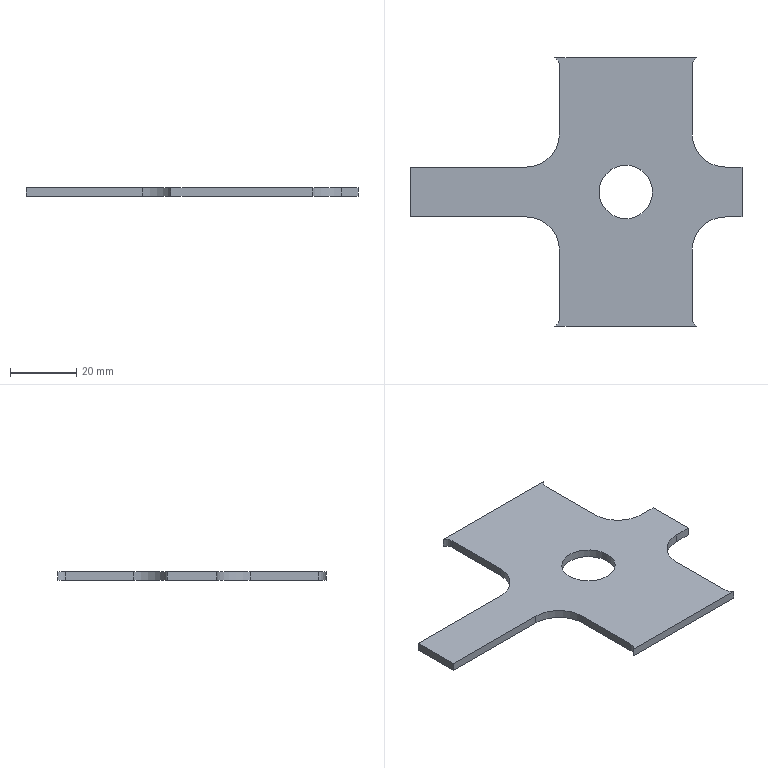Part | STEP file | lll_id1202_x_t | 1 solid | 23 faces | box 100 x 81 x 2.5 mm | volume 10066 mm3 | plane 14 | cylinder 9 | commonest cylinder face diameters 6 x4 20 x4 16.1 x1
STEP:
#1=CARTESIAN_POINT('',(3841.,38.,0.));
#2=VERTEX_POINT('',#1);
#3=CARTESIAN_POINT('',(3841.,17.5,0.));
#4=VERTEX_POINT('',#3);
#5=CARTESIAN_POINT('',(3841.,38.,0.));
#6=DIRECTION('',(0.,-1.,0.));
#7=VECTOR('',#6,1.);
#8=LINE('',#5,#7);
#9=EDGE_CURVE('',#2,#4,#8,.T.);
#10=ORIENTED_EDGE('',*,*,#9,.T.);
#11=CARTESIAN_POINT('',(3841.,17.5,2.5));
#12=VERTEX_POINT('',#11);
#13=CARTESIAN_POINT('',(3841.,17.5,2.5));
#14=DIRECTION('',(0.,0.,1.));
#15=VECTOR('',#14,1.);
#16=LINE('',#13,#15);
#17=EDGE_CURVE('',#4,#12,#16,.T.);
#18=ORIENTED_EDGE('',*,*,#17,.T.);
#19=CARTESIAN_POINT('',(3841.,38.,2.5));
#20=VERTEX_POINT('',#19);
#21=CARTESIAN_POINT('',(3841.,38.,2.5));
#22=DIRECTION('',(0.,-1.,0.));
#23=VECTOR('',#22,1.);
#24=LINE('',#21,#23);
#25=EDGE_CURVE('',#20,#12,#24,.T.);
#26=ORIENTED_EDGE('',*,*,#25,.F.);
#27=CARTESIAN_POINT('',(3841.,38.,2.5));
#28=DIRECTION('',(0.,0.,1.));
#29=VECTOR('',#28,1.);
#30=LINE('',#27,#29);
#31=EDGE_CURVE('',#2,#20,#30,.T.);
#32=ORIENTED_EDGE('',*,*,#31,.F.);
#33=EDGE_LOOP('',(#10,#18,#26,#32));
#34=FACE_OUTER_BOUND('',#33,.T.);
#35=CARTESIAN_POINT('',(3841.,38.,2.5));
#36=DIRECTION('',(1.,0.,0.));
#37=DIRECTION('',(0.,0.,-1.));
#38=AXIS2_PLACEMENT_3D('',#35,#36,#37);
#39=PLANE('',#38);
#40=ADVANCED_FACE('',(#34),#39,.F.);
#41=CARTESIAN_POINT('',(3839.658,40.5,2.5));
#42=VERTEX_POINT('',#41);
#43=CARTESIAN_POINT('',(3838.,38.,2.5));
#44=DIRECTION('',(0.,0.,-1.));
#45=DIRECTION('',(-1.,0.,0.));
#46=AXIS2_PLACEMENT_3D('',#43,#44,#45);
#47=CIRCLE('',#46,3.);
#48=EDGE_CURVE('',#42,#20,#47,.T.);
#49=ORIENTED_EDGE('',*,*,#48,.F.);
#50=CARTESIAN_POINT('',(3839.658,40.5,0.));
#51=VERTEX_POINT('',#50);
#52=CARTESIAN_POINT('',(3839.658,40.5,1.25));
#53=DIRECTION('',(-0.000000011,0.000000008,-1.));
#54=VECTOR('',#53,1.);
#55=LINE('',#52,#54);
#56=EDGE_CURVE('',#42,#51,#55,.T.);
#57=ORIENTED_EDGE('',*,*,#56,.T.);
#58=CARTESIAN_POINT('',(3838.,38.,0.));
#59=DIRECTION('',(0.,0.,-1.));
#60=DIRECTION('',(-1.,0.,0.));
#61=AXIS2_PLACEMENT_3D('',#58,#59,#60);
#62=CIRCLE('',#61,3.);
#63=EDGE_CURVE('',#51,#2,#62,.T.);
#64=ORIENTED_EDGE('',*,*,#63,.T.);
#65=ORIENTED_EDGE('',*,*,#31,.T.);
#66=EDGE_LOOP('',(#49,#57,#64,#65));
#67=FACE_OUTER_BOUND('',#66,.T.);
#68=CARTESIAN_POINT('',(3838.,38.,2.5));
#69=DIRECTION('',(0.,0.,-1.));
#70=DIRECTION('',(-1.,0.,0.));
#71=AXIS2_PLACEMENT_3D('',#68,#69,#70);
#72=CYLINDRICAL_SURFACE('',#71,3.);
#73=ADVANCED_FACE('',(#67),#72,.F.);
#74=CARTESIAN_POINT('',(3882.342,40.5,2.5));
#75=VERTEX_POINT('',#74);
#76=CARTESIAN_POINT('',(3882.342,40.5,-0.000000212));
#77=VERTEX_POINT('',#76);
#78=CARTESIAN_POINT('',(3882.342,40.5,1.25));
#79=DIRECTION('',(0.000000011,0.000000008,-1.));
#80=VECTOR('',#79,1.);
#81=LINE('',#78,#80);
#82=EDGE_CURVE('',#75,#77,#81,.T.);
#83=ORIENTED_EDGE('',*,*,#82,.T.);
#84=CARTESIAN_POINT('',(14362.883,40.5,0.));
#85=DIRECTION('',(-1.,0.,0.));
#86=VECTOR('',#85,1.);
#87=LINE('',#84,#86);
#88=EDGE_CURVE('',#77,#51,#87,.T.);
#89=ORIENTED_EDGE('',*,*,#88,.T.);
#90=ORIENTED_EDGE('',*,*,#56,.F.);
#91=CARTESIAN_POINT('',(14362.883,40.5,2.5));
#92=DIRECTION('',(1.,0.,0.));
#93=VECTOR('',#92,1.);
#94=LINE('',#91,#93);
#95=EDGE_CURVE('',#42,#75,#94,.T.);
#96=ORIENTED_EDGE('',*,*,#95,.T.);
#97=EDGE_LOOP('',(#83,#89,#90,#96));
#98=FACE_OUTER_BOUND('',#97,.T.);
#99=CARTESIAN_POINT('',(3821.426,40.5,2.5));
#100=DIRECTION('',(0.,-1.,-0.000000008));
#101=DIRECTION('',(0.,-0.000000008,1.));
#102=AXIS2_PLACEMENT_3D('',#99,#100,#101);
#103=PLANE('',#102);
#104=ADVANCED_FACE('',(#98),#103,.F.);
#105=ORIENTED_EDGE('',*,*,#82,.F.);
#106=CARTESIAN_POINT('',(3881.,38.,2.5));
#107=VERTEX_POINT('',#106);
#108=CARTESIAN_POINT('',(3884.,38.,2.5));
#109=DIRECTION('',(0.,0.,1.));
#110=DIRECTION('',(-1.,0.,0.));
#111=AXIS2_PLACEMENT_3D('',#108,#109,#110);
#112=CIRCLE('',#111,3.);
#113=EDGE_CURVE('',#75,#107,#112,.T.);
#114=ORIENTED_EDGE('',*,*,#113,.T.);
#115=CARTESIAN_POINT('',(3881.,38.,0.));
#116=VERTEX_POINT('',#115);
#117=CARTESIAN_POINT('',(3881.,38.,2.5));
#118=DIRECTION('',(0.,0.,1.));
#119=VECTOR('',#118,1.);
#120=LINE('',#117,#119);
#121=EDGE_CURVE('',#116,#107,#120,.T.);
#122=ORIENTED_EDGE('',*,*,#121,.F.);
#123=CARTESIAN_POINT('',(3884.,38.,0.));
#124=DIRECTION('',(0.,0.,1.));
#125=DIRECTION('',(-1.,0.,0.));
#126=AXIS2_PLACEMENT_3D('',#123,#124,#125);
#127=CIRCLE('',#126,3.);
#128=EDGE_CURVE('',#77,#116,#127,.T.);
#129=ORIENTED_EDGE('',*,*,#128,.F.);
#130=EDGE_LOOP('',(#105,#114,#122,#129));
#131=FACE_OUTER_BOUND('',#130,.T.);
#132=CARTESIAN_POINT('',(3884.,38.,2.5));
#133=DIRECTION('',(0.,0.,-1.));
#134=DIRECTION('',(-1.,0.,0.));
#135=AXIS2_PLACEMENT_3D('',#132,#133,#134);
#136=CYLINDRICAL_SURFACE('',#135,3.);
#137=ADVANCED_FACE('',(#131),#136,.F.);
#138=CARTESIAN_POINT('',(3881.,17.5,0.));
#139=VERTEX_POINT('',#138);
#140=CARTESIAN_POINT('',(3881.,38.,0.));
#141=DIRECTION('',(0.,-1.,0.));
#142=VECTOR('',#141,1.);
#143=LINE('',#140,#142);
#144=EDGE_CURVE('',#116,#139,#143,.T.);
#145=ORIENTED_EDGE('',*,*,#144,.F.);
#146=ORIENTED_EDGE('',*,*,#121,.T.);
#147=CARTESIAN_POINT('',(3881.,17.5,2.5));
#148=VERTEX_POINT('',#147);
#149=CARTESIAN_POINT('',(3881.,38.,2.5));
#150=DIRECTION('',(0.,-1.,0.));
#151=VECTOR('',#150,1.);
#152=LINE('',#149,#151);
#153=EDGE_CURVE('',#107,#148,#152,.T.);
#154=ORIENTED_EDGE('',*,*,#153,.T.);
#155=CARTESIAN_POINT('',(3881.,17.5,2.5));
#156=DIRECTION('',(0.,0.,1.));
#157=VECTOR('',#156,1.);
#158=LINE('',#155,#157);
#159=EDGE_CURVE('',#139,#148,#158,.T.);
#160=ORIENTED_EDGE('',*,*,#159,.F.);
#161=EDGE_LOOP('',(#145,#146,#154,#160));
#162=FACE_OUTER_BOUND('',#161,.T.);
#163=CARTESIAN_POINT('',(3881.,38.,2.5));
#164=DIRECTION('',(1.,0.,0.));
#165=DIRECTION('',(0.,0.,-1.));
#166=AXIS2_PLACEMENT_3D('',#163,#164,#165);
#167=PLANE('',#166);
#168=ADVANCED_FACE('',(#162),#167,.T.);
#169=CARTESIAN_POINT('',(3891.,7.5,0.));
#170=VERTEX_POINT('',#169);
#171=CARTESIAN_POINT('',(3891.,17.5,0.));
#172=DIRECTION('',(0.,0.,1.));
#173=DIRECTION('',(-1.,0.,0.));
#174=AXIS2_PLACEMENT_3D('',#171,#172,#173);
#175=CIRCLE('',#174,10.);
#176=EDGE_CURVE('',#139,#170,#175,.T.);
#177=ORIENTED_EDGE('',*,*,#176,.F.);
#178=ORIENTED_EDGE('',*,*,#159,.T.);
#179=CARTESIAN_POINT('',(3891.,7.5,2.5));
#180=VERTEX_POINT('',#179);
#181=CARTESIAN_POINT('',(3891.,17.5,2.5));
#182=DIRECTION('',(0.,0.,1.));
#183=DIRECTION('',(-1.,0.,0.));
#184=AXIS2_PLACEMENT_3D('',#181,#182,#183);
#185=CIRCLE('',#184,10.);
#186=EDGE_CURVE('',#148,#180,#185,.T.);
#187=ORIENTED_EDGE('',*,*,#186,.T.);
#188=CARTESIAN_POINT('',(3891.,7.5,2.5));
#189=DIRECTION('',(0.,0.,1.));
#190=VECTOR('',#189,1.);
#191=LINE('',#188,#190);
#192=EDGE_CURVE('',#170,#180,#191,.T.);
#193=ORIENTED_EDGE('',*,*,#192,.F.);
#194=EDGE_LOOP('',(#177,#178,#187,#193));
#195=FACE_OUTER_BOUND('',#194,.T.);
#196=CARTESIAN_POINT('',(3891.,17.5,2.5));
#197=DIRECTION('',(0.,0.,-1.));
#198=DIRECTION('',(-1.,0.,0.));
#199=AXIS2_PLACEMENT_3D('',#196,#197,#198);
#200=CYLINDRICAL_SURFACE('',#199,10.);
#201=ADVANCED_FACE('',(#195),#200,.F.);
#202=CARTESIAN_POINT('',(3896.,7.5,0.));
#203=VERTEX_POINT('',#202);
#204=CARTESIAN_POINT('',(3896.,7.5,2.5));
#205=VERTEX_POINT('',#204);
#206=CARTESIAN_POINT('',(3896.,7.5,2.5));
#207=DIRECTION('',(0.,0.,1.));
#208=VECTOR('',#207,1.);
#209=LINE('',#206,#208);
#210=EDGE_CURVE('',#203,#205,#209,.T.);
#211=ORIENTED_EDGE('',*,*,#210,.F.);
#212=CARTESIAN_POINT('',(3891.,7.5,0.));
#213=DIRECTION('',(1.,0.,0.));
#214=VECTOR('',#213,1.);
#215=LINE('',#212,#214);
#216=EDGE_CURVE('',#170,#203,#215,.T.);
#217=ORIENTED_EDGE('',*,*,#216,.F.);
#218=ORIENTED_EDGE('',*,*,#192,.T.);
#219=CARTESIAN_POINT('',(3891.,7.5,2.5));
#220=DIRECTION('',(1.,0.,0.));
#221=VECTOR('',#220,1.);
#222=LINE('',#219,#221);
#223=EDGE_CURVE('',#180,#205,#222,.T.);
#224=ORIENTED_EDGE('',*,*,#223,.T.);
#225=EDGE_LOOP('',(#211,#217,#218,#224));
#226=FACE_OUTER_BOUND('',#225,.T.);
#227=CARTESIAN_POINT('',(3891.,7.5,2.5));
#228=DIRECTION('',(0.,1.,0.));
#229=DIRECTION('',(0.,0.,1.));
#230=AXIS2_PLACEMENT_3D('',#227,#228,#229);
#231=PLANE('',#230);
#232=ADVANCED_FACE('',(#226),#231,.T.);
#233=CARTESIAN_POINT('',(3896.,-7.5,0.));
#234=VERTEX_POINT('',#233);
#235=CARTESIAN_POINT('',(3896.,-13712.786,0.));
#236=DIRECTION('',(0.,1.,0.));
#237=VECTOR('',#236,1.);
#238=LINE('',#235,#237);
#239=EDGE_CURVE('',#234,#203,#238,.T.);
#240=ORIENTED_EDGE('',*,*,#239,.T.);
#241=ORIENTED_EDGE('',*,*,#210,.T.);
#242=CARTESIAN_POINT('',(3896.,-7.5,2.5));
#243=VERTEX_POINT('',#242);
#244=CARTESIAN_POINT('',(3896.,-13712.786,2.5));
#245=DIRECTION('',(0.,-1.,0.));
#246=VECTOR('',#245,1.);
#247=LINE('',#244,#246);
#248=EDGE_CURVE('',#205,#243,#247,.T.);
#249=ORIENTED_EDGE('',*,*,#248,.T.);
#250=CARTESIAN_POINT('',(3896.,-7.5,2.5));
#251=DIRECTION('',(0.,0.,-1.));
#252=VECTOR('',#251,1.);
#253=LINE('',#250,#252);
#254=EDGE_CURVE('',#243,#234,#253,.T.);
#255=ORIENTED_EDGE('',*,*,#254,.T.);
#256=EDGE_LOOP('',(#240,#241,#249,#255));
#257=FACE_OUTER_BOUND('',#256,.T.);
#258=CARTESIAN_POINT('',(3896.,29.64,-1302.5));
#259=DIRECTION('',(-1.,0.,0.));
#260=DIRECTION('',(0.,0.,1.));
#261=AXIS2_PLACEMENT_3D('',#258,#259,#260);
#262=PLANE('',#261);
#263=ADVANCED_FACE('',(#257),#262,.F.);
#264=ORIENTED_EDGE('',*,*,#254,.F.);
#265=CARTESIAN_POINT('',(3891.,-7.5,2.5));
#266=VERTEX_POINT('',#265);
#267=CARTESIAN_POINT('',(3973.,-7.5,2.5));
#268=DIRECTION('',(-1.,0.,0.));
#269=VECTOR('',#268,1.);
#270=LINE('',#267,#269);
#271=EDGE_CURVE('',#243,#266,#270,.T.);
#272=ORIENTED_EDGE('',*,*,#271,.T.);
#273=CARTESIAN_POINT('',(3891.,-7.5,0.));
#274=VERTEX_POINT('',#273);
#275=CARTESIAN_POINT('',(3891.,-7.5,2.5));
#276=DIRECTION('',(0.,0.,1.));
#277=VECTOR('',#276,1.);
#278=LINE('',#275,#277);
#279=EDGE_CURVE('',#274,#266,#278,.T.);
#280=ORIENTED_EDGE('',*,*,#279,.F.);
#281=CARTESIAN_POINT('',(3973.,-7.5,0.));
#282=DIRECTION('',(-1.,0.,0.));
#283=VECTOR('',#282,1.);
#284=LINE('',#281,#283);
#285=EDGE_CURVE('',#234,#274,#284,.T.);
#286=ORIENTED_EDGE('',*,*,#285,.F.);
#287=EDGE_LOOP('',(#264,#272,#280,#286));
#288=FACE_OUTER_BOUND('',#287,.T.);
#289=CARTESIAN_POINT('',(3973.,-7.5,2.5));
#290=DIRECTION('',(0.,-1.,0.));
#291=DIRECTION('',(0.,0.,-1.));
#292=AXIS2_PLACEMENT_3D('',#289,#290,#291);
#293=PLANE('',#292);
#294=ADVANCED_FACE('',(#288),#293,.T.);
#295=CARTESIAN_POINT('',(3881.,-17.5,0.));
#296=VERTEX_POINT('',#295);
#297=CARTESIAN_POINT('',(3891.,-17.5,0.));
#298=DIRECTION('',(0.,0.,1.));
#299=DIRECTION('',(-1.,0.,0.));
#300=AXIS2_PLACEMENT_3D('',#297,#298,#299);
#301=CIRCLE('',#300,10.);
#302=EDGE_CURVE('',#274,#296,#301,.T.);
#303=ORIENTED_EDGE('',*,*,#302,.F.);
#304=ORIENTED_EDGE('',*,*,#279,.T.);
#305=CARTESIAN_POINT('',(3881.,-17.5,2.5));
#306=VERTEX_POINT('',#305);
#307=CARTESIAN_POINT('',(3891.,-17.5,2.5));
#308=DIRECTION('',(0.,0.,1.));
#309=DIRECTION('',(-1.,0.,0.));
#310=AXIS2_PLACEMENT_3D('',#307,#308,#309);
#311=CIRCLE('',#310,10.);
#312=EDGE_CURVE('',#266,#306,#311,.T.);
#313=ORIENTED_EDGE('',*,*,#312,.T.);
#314=CARTESIAN_POINT('',(3881.,-17.5,2.5));
#315=DIRECTION('',(0.,0.,1.));
#316=VECTOR('',#315,1.);
#317=LINE('',#314,#316);
#318=EDGE_CURVE('',#296,#306,#317,.T.);
#319=ORIENTED_EDGE('',*,*,#318,.F.);
#320=EDGE_LOOP('',(#303,#304,#313,#319));
#321=FACE_OUTER_BOUND('',#320,.T.);
#322=CARTESIAN_POINT('',(3891.,-17.5,2.5));
#323=DIRECTION('',(0.,0.,-1.));
#324=DIRECTION('',(-1.,0.,0.));
#325=AXIS2_PLACEMENT_3D('',#322,#323,#324);
#326=CYLINDRICAL_SURFACE('',#325,10.);
#327=ADVANCED_FACE('',(#321),#326,.F.);
#328=CARTESIAN_POINT('',(3881.,-38.,0.));
#329=VERTEX_POINT('',#328);
#330=CARTESIAN_POINT('',(3881.,-17.5,0.));
#331=DIRECTION('',(0.,-1.,0.));
#332=VECTOR('',#331,1.);
#333=LINE('',#330,#332);
#334=EDGE_CURVE('',#296,#329,#333,.T.);
#335=ORIENTED_EDGE('',*,*,#334,.F.);
#336=ORIENTED_EDGE('',*,*,#318,.T.);
#337=CARTESIAN_POINT('',(3881.,-38.,2.5));
#338=VERTEX_POINT('',#337);
#339=CARTESIAN_POINT('',(3881.,-17.5,2.5));
#340=DIRECTION('',(0.,-1.,0.));
#341=VECTOR('',#340,1.);
#342=LINE('',#339,#341);
#343=EDGE_CURVE('',#306,#338,#342,.T.);
#344=ORIENTED_EDGE('',*,*,#343,.T.);
#345=CARTESIAN_POINT('',(3881.,-38.,2.5));
#346=DIRECTION('',(0.,0.,1.));
#347=VECTOR('',#346,1.);
#348=LINE('',#345,#347);
#349=EDGE_CURVE('',#329,#338,#348,.T.);
#350=ORIENTED_EDGE('',*,*,#349,.F.);
#351=EDGE_LOOP('',(#335,#336,#344,#350));
#352=FACE_OUTER_BOUND('',#351,.T.);
#353=CARTESIAN_POINT('',(3881.,-17.5,2.5));
#354=DIRECTION('',(1.,0.,0.));
#355=DIRECTION('',(0.,0.,-1.));
#356=AXIS2_PLACEMENT_3D('',#353,#354,#355);
#357=PLANE('',#356);
#358=ADVANCED_FACE('',(#352),#357,.T.);
#359=CARTESIAN_POINT('',(3882.342,-40.5,2.5));
#360=VERTEX_POINT('',#359);
#361=CARTESIAN_POINT('',(3882.342,-40.5,-0.000001069));
#362=VERTEX_POINT('',#361);
#363=CARTESIAN_POINT('',(3882.342,-40.5,2.5));
#364=DIRECTION('',(0.,0.,-1.));
#365=VECTOR('',#364,1.);
#366=LINE('',#363,#365);
#367=EDGE_CURVE('',#360,#362,#366,.T.);
#368=ORIENTED_EDGE('',*,*,#367,.T.);
#369=CARTESIAN_POINT('',(3884.,-38.,0.));
#370=DIRECTION('',(0.,0.,1.));
#371=DIRECTION('',(-1.,0.,0.));
#372=AXIS2_PLACEMENT_3D('',#369,#370,#371);
#373=CIRCLE('',#372,3.);
#374=EDGE_CURVE('',#329,#362,#373,.T.);
#375=ORIENTED_EDGE('',*,*,#374,.F.);
#376=ORIENTED_EDGE('',*,*,#349,.T.);
#377=CARTESIAN_POINT('',(3884.,-38.,2.5));
#378=DIRECTION('',(0.,0.,1.));
#379=DIRECTION('',(-1.,0.,0.));
#380=AXIS2_PLACEMENT_3D('',#377,#378,#379);
#381=CIRCLE('',#380,3.);
#382=EDGE_CURVE('',#338,#360,#381,.T.);
#383=ORIENTED_EDGE('',*,*,#382,.T.);
#384=EDGE_LOOP('',(#368,#375,#376,#383));
#385=FACE_OUTER_BOUND('',#384,.T.);
#386=CARTESIAN_POINT('',(3884.,-38.,2.5));
#387=DIRECTION('',(0.,0.,-1.));
#388=DIRECTION('',(-1.,0.,0.));
#389=AXIS2_PLACEMENT_3D('',#386,#387,#388);
#390=CYLINDRICAL_SURFACE('',#389,3.);
#391=ADVANCED_FACE('',(#385),#390,.F.);
#392=ORIENTED_EDGE('',*,*,#367,.F.);
#393=CARTESIAN_POINT('',(3839.658,-40.5,2.5));
#394=VERTEX_POINT('',#393);
#395=CARTESIAN_POINT('',(14362.883,-40.5,2.5));
#396=DIRECTION('',(1.,0.,0.));
#397=VECTOR('',#396,1.);
#398=LINE('',#395,#397);
#399=EDGE_CURVE('',#394,#360,#398,.T.);
#400=ORIENTED_EDGE('',*,*,#399,.F.);
#401=CARTESIAN_POINT('',(3839.658,-40.5,-0.000001393));
#402=VERTEX_POINT('',#401);
#403=CARTESIAN_POINT('',(3839.658,-40.5,2.5));
#404=DIRECTION('',(0.,0.,1.));
#405=VECTOR('',#404,1.);
#406=LINE('',#403,#405);
#407=EDGE_CURVE('',#402,#394,#406,.T.);
#408=ORIENTED_EDGE('',*,*,#407,.F.);
#409=CARTESIAN_POINT('',(14362.883,-40.5,0.));
#410=DIRECTION('',(1.,0.,0.));
#411=VECTOR('',#410,1.);
#412=LINE('',#409,#411);
#413=EDGE_CURVE('',#402,#362,#412,.T.);
#414=ORIENTED_EDGE('',*,*,#413,.T.);
#415=EDGE_LOOP('',(#392,#400,#408,#414));
#416=FACE_OUTER_BOUND('',#415,.T.);
#417=CARTESIAN_POINT('',(3821.426,-40.5,-0.000001531));
#418=DIRECTION('',(0.,1.,0.));
#419=DIRECTION('',(0.000000008,0.,-1.));
#420=AXIS2_PLACEMENT_3D('',#417,#418,#419);
#421=PLANE('',#420);
#422=ADVANCED_FACE('',(#416),#421,.F.);
#423=ORIENTED_EDGE('',*,*,#407,.T.);
#424=CARTESIAN_POINT('',(3841.,-38.,2.5));
#425=VERTEX_POINT('',#424);
#426=CARTESIAN_POINT('',(3838.,-38.,2.5));
#427=DIRECTION('',(0.,0.,1.));
#428=DIRECTION('',(-1.,0.,0.));
#429=AXIS2_PLACEMENT_3D('',#426,#427,#428);
#430=CIRCLE('',#429,3.);
#431=EDGE_CURVE('',#394,#425,#430,.T.);
#432=ORIENTED_EDGE('',*,*,#431,.T.);
#433=CARTESIAN_POINT('',(3841.,-38.,0.));
#434=VERTEX_POINT('',#433);
#435=CARTESIAN_POINT('',(3841.,-38.,2.5));
#436=DIRECTION('',(0.,0.,1.));
#437=VECTOR('',#436,1.);
#438=LINE('',#435,#437);
#439=EDGE_CURVE('',#434,#425,#438,.T.);
#440=ORIENTED_EDGE('',*,*,#439,.F.);
#441=CARTESIAN_POINT('',(3838.,-38.,0.));
#442=DIRECTION('',(0.,0.,1.));
#443=DIRECTION('',(-1.,0.,0.));
#444=AXIS2_PLACEMENT_3D('',#441,#442,#443);
#445=CIRCLE('',#444,3.);
#446=EDGE_CURVE('',#402,#434,#445,.T.);
#447=ORIENTED_EDGE('',*,*,#446,.F.);
#448=EDGE_LOOP('',(#423,#432,#440,#447));
#449=FACE_OUTER_BOUND('',#448,.T.);
#450=CARTESIAN_POINT('',(3838.,-38.,2.5));
#451=DIRECTION('',(0.,0.,-1.));
#452=DIRECTION('',(-1.,0.,0.));
#453=AXIS2_PLACEMENT_3D('',#450,#451,#452);
#454=CYLINDRICAL_SURFACE('',#453,3.);
#455=ADVANCED_FACE('',(#449),#454,.F.);
#456=CARTESIAN_POINT('',(3841.,-17.5,0.));
#457=VERTEX_POINT('',#456);
#458=CARTESIAN_POINT('',(3841.,-38.,0.));
#459=DIRECTION('',(0.,1.,0.));
#460=VECTOR('',#459,1.);
#461=LINE('',#458,#460);
#462=EDGE_CURVE('',#434,#457,#461,.T.);
#463=ORIENTED_EDGE('',*,*,#462,.F.);
#464=ORIENTED_EDGE('',*,*,#439,.T.);
#465=CARTESIAN_POINT('',(3841.,-17.5,2.5));
#466=VERTEX_POINT('',#465);
#467=CARTESIAN_POINT('',(3841.,-38.,2.5));
#468=DIRECTION('',(0.,1.,0.));
#469=VECTOR('',#468,1.);
#470=LINE('',#467,#469);
#471=EDGE_CURVE('',#425,#466,#470,.T.);
#472=ORIENTED_EDGE('',*,*,#471,.T.);
#473=CARTESIAN_POINT('',(3841.,-17.5,2.5));
#474=DIRECTION('',(0.,0.,1.));
#475=VECTOR('',#474,1.);
#476=LINE('',#473,#475);
#477=EDGE_CURVE('',#457,#466,#476,.T.);
#478=ORIENTED_EDGE('',*,*,#477,.F.);
#479=EDGE_LOOP('',(#463,#464,#472,#478));
#480=FACE_OUTER_BOUND('',#479,.T.);
#481=CARTESIAN_POINT('',(3841.,-38.,2.5));
#482=DIRECTION('',(-1.,0.,0.));
#483=DIRECTION('',(0.,1.,0.));
#484=AXIS2_PLACEMENT_3D('',#481,#482,#483);
#485=PLANE('',#484);
#486=ADVANCED_FACE('',(#480),#485,.T.);
#487=CARTESIAN_POINT('',(3852.95,0.,2.5));
#488=VERTEX_POINT('',#487);
#489=CARTESIAN_POINT('',(3861.,0.,2.5));
#490=DIRECTION('',(0.,0.,1.));
#491=DIRECTION('',(-1.,0.,0.));
#492=AXIS2_PLACEMENT_3D('',#489,#490,#491);
#493=CIRCLE('',#492,8.05);
#494=EDGE_CURVE('',#488,#488,#493,.T.);
#495=ORIENTED_EDGE('',*,*,#494,.T.);
#496=EDGE_LOOP('',(#495));
#497=FACE_BOUND('',#496,.T.);
#498=CARTESIAN_POINT('',(3852.95,0.,0.));
#499=VERTEX_POINT('',#498);
#500=CARTESIAN_POINT('',(3861.,0.,0.));
#501=DIRECTION('',(0.,0.,1.));
#502=DIRECTION('',(-1.,0.,0.));
#503=AXIS2_PLACEMENT_3D('',#500,#501,#502);
#504=CIRCLE('',#503,8.05);
#505=EDGE_CURVE('',#499,#499,#504,.T.);
#506=ORIENTED_EDGE('',*,*,#505,.F.);
#507=EDGE_LOOP('',(#506));
#508=FACE_BOUND('',#507,.T.);
#509=CARTESIAN_POINT('',(3861.,0.,2.5));
#510=DIRECTION('',(0.,0.,-1.));
#511=DIRECTION('',(-1.,0.,0.));
#512=AXIS2_PLACEMENT_3D('',#509,#510,#511);
#513=CYLINDRICAL_SURFACE('',#512,8.05);
#514=ADVANCED_FACE('',(#497,#508),#513,.F.);
#515=CARTESIAN_POINT('',(3831.,-7.5,0.));
#516=VERTEX_POINT('',#515);
#517=CARTESIAN_POINT('',(3831.,-17.5,0.));
#518=DIRECTION('',(0.,0.,1.));
#519=DIRECTION('',(-1.,0.,0.));
#520=AXIS2_PLACEMENT_3D('',#517,#518,#519);
#521=CIRCLE('',#520,10.);
#522=EDGE_CURVE('',#457,#516,#521,.T.);
#523=ORIENTED_EDGE('',*,*,#522,.F.);
#524=ORIENTED_EDGE('',*,*,#477,.T.);
#525=CARTESIAN_POINT('',(3831.,-7.5,2.5));
#526=VERTEX_POINT('',#525);
#527=CARTESIAN_POINT('',(3831.,-17.5,2.5));
#528=DIRECTION('',(0.,0.,1.));
#529=DIRECTION('',(-1.,0.,0.));
#530=AXIS2_PLACEMENT_3D('',#527,#528,#529);
#531=CIRCLE('',#530,10.);
#532=EDGE_CURVE('',#466,#526,#531,.T.);
#533=ORIENTED_EDGE('',*,*,#532,.T.);
#534=CARTESIAN_POINT('',(3831.,-7.5,2.5));
#535=DIRECTION('',(0.,0.,1.));
#536=VECTOR('',#535,1.);
#537=LINE('',#534,#536);
#538=EDGE_CURVE('',#516,#526,#537,.T.);
#539=ORIENTED_EDGE('',*,*,#538,.F.);
#540=EDGE_LOOP('',(#523,#524,#533,#539));
#541=FACE_OUTER_BOUND('',#540,.T.);
#542=CARTESIAN_POINT('',(3831.,-17.5,2.5));
#543=DIRECTION('',(0.,0.,-1.));
#544=DIRECTION('',(-1.,0.,0.));
#545=AXIS2_PLACEMENT_3D('',#542,#543,#544);
#546=CYLINDRICAL_SURFACE('',#545,10.);
#547=ADVANCED_FACE('',(#541),#546,.F.);
#548=CARTESIAN_POINT('',(3831.,7.5,0.));
#549=VERTEX_POINT('',#548);
#550=CARTESIAN_POINT('',(3831.,17.5,0.));
#551=DIRECTION('',(0.,0.,-1.));
#552=DIRECTION('',(-1.,0.,0.));
#553=AXIS2_PLACEMENT_3D('',#550,#551,#552);
#554=CIRCLE('',#553,10.);
#555=EDGE_CURVE('',#4,#549,#554,.T.);
#556=ORIENTED_EDGE('',*,*,#555,.T.);
#557=CARTESIAN_POINT('',(3831.,7.5,2.5));
#558=VERTEX_POINT('',#557);
#559=CARTESIAN_POINT('',(3831.,7.5,2.5));
#560=DIRECTION('',(0.,0.,1.));
#561=VECTOR('',#560,1.);
#562=LINE('',#559,#561);
#563=EDGE_CURVE('',#549,#558,#562,.T.);
#564=ORIENTED_EDGE('',*,*,#563,.T.);
#565=CARTESIAN_POINT('',(3831.,17.5,2.5));
#566=DIRECTION('',(0.,0.,-1.));
#567=DIRECTION('',(-1.,0.,0.));
#568=AXIS2_PLACEMENT_3D('',#565,#566,#567);
#569=CIRCLE('',#568,10.);
#570=EDGE_CURVE('',#12,#558,#569,.T.);
#571=ORIENTED_EDGE('',*,*,#570,.F.);
#572=ORIENTED_EDGE('',*,*,#17,.F.);
#573=EDGE_LOOP('',(#556,#564,#571,#572));
#574=FACE_OUTER_BOUND('',#573,.T.);
#575=CARTESIAN_POINT('',(3831.,17.5,2.5));
#576=DIRECTION('',(0.,0.,-1.));
#577=DIRECTION('',(-1.,0.,0.));
#578=AXIS2_PLACEMENT_3D('',#575,#576,#577);
#579=CYLINDRICAL_SURFACE('',#578,10.);
#580=ADVANCED_FACE('',(#574),#579,.F.);
#581=CARTESIAN_POINT('',(3796.,-7.5,2.5));
#582=VERTEX_POINT('',#581);
#583=CARTESIAN_POINT('',(3796.,-7.5,0.));
#584=VERTEX_POINT('',#583);
#585=CARTESIAN_POINT('',(3796.,-7.5,2.5));
#586=DIRECTION('',(0.,0.,-1.));
#587=VECTOR('',#586,1.);
#588=LINE('',#585,#587);
#589=EDGE_CURVE('',#582,#584,#588,.T.);
#590=ORIENTED_EDGE('',*,*,#589,.T.);
#591=CARTESIAN_POINT('',(3831.,-7.5,0.));
#592=DIRECTION('',(-1.,0.,0.));
#593=VECTOR('',#592,1.);
#594=LINE('',#591,#593);
#595=EDGE_CURVE('',#516,#584,#594,.T.);
#596=ORIENTED_EDGE('',*,*,#595,.F.);
#597=ORIENTED_EDGE('',*,*,#538,.T.);
#598=CARTESIAN_POINT('',(3831.,-7.5,2.5));
#599=DIRECTION('',(-1.,0.,0.));
#600=VECTOR('',#599,1.);
#601=LINE('',#598,#600);
#602=EDGE_CURVE('',#526,#582,#601,.T.);
#603=ORIENTED_EDGE('',*,*,#602,.T.);
#604=EDGE_LOOP('',(#590,#596,#597,#603));
#605=FACE_OUTER_BOUND('',#604,.T.);
#606=CARTESIAN_POINT('',(3831.,-7.5,2.5));
#607=DIRECTION('',(0.,-1.,0.));
#608=DIRECTION('',(-1.,0.,0.));
#609=AXIS2_PLACEMENT_3D('',#606,#607,#608);
#610=PLANE('',#609);
#611=ADVANCED_FACE('',(#605),#610,.T.);
#612=CARTESIAN_POINT('',(3796.,7.5,0.));
#613=VERTEX_POINT('',#612);
#614=CARTESIAN_POINT('',(3831.,7.5,0.));
#615=DIRECTION('',(-1.,0.,0.));
#616=VECTOR('',#615,1.);
#617=LINE('',#614,#616);
#618=EDGE_CURVE('',#549,#613,#617,.T.);
#619=ORIENTED_EDGE('',*,*,#618,.T.);
#620=CARTESIAN_POINT('',(3796.,7.5,2.5));
#621=VERTEX_POINT('',#620);
#622=CARTESIAN_POINT('',(3796.,7.5,2.5));
#623=DIRECTION('',(0.,0.,1.));
#624=VECTOR('',#623,1.);
#625=LINE('',#622,#624);
#626=EDGE_CURVE('',#613,#621,#625,.T.);
#627=ORIENTED_EDGE('',*,*,#626,.T.);
#628=CARTESIAN_POINT('',(3831.,7.5,2.5));
#629=DIRECTION('',(-1.,0.,0.));
#630=VECTOR('',#629,1.);
#631=LINE('',#628,#630);
#632=EDGE_CURVE('',#558,#621,#631,.T.);
#633=ORIENTED_EDGE('',*,*,#632,.F.);
#634=ORIENTED_EDGE('',*,*,#563,.F.);
#635=EDGE_LOOP('',(#619,#627,#633,#634));
#636=FACE_OUTER_BOUND('',#635,.T.);
#637=CARTESIAN_POINT('',(3831.,7.5,2.5));
#638=DIRECTION('',(0.,-1.,0.));
#639=DIRECTION('',(-1.,0.,0.));
#640=AXIS2_PLACEMENT_3D('',#637,#638,#639);
#641=PLANE('',#640);
#642=ADVANCED_FACE('',(#636),#641,.F.);
#643=ORIENTED_EDGE('',*,*,#494,.F.);
#644=EDGE_LOOP('',(#643));
#645=FACE_BOUND('',#644,.T.);
#646=ORIENTED_EDGE('',*,*,#632,.T.);
#647=CARTESIAN_POINT('',(3796.,-13712.786,2.5));
#648=DIRECTION('',(0.,1.,0.));
#649=VECTOR('',#648,1.);
#650=LINE('',#647,#649);
#651=EDGE_CURVE('',#582,#621,#650,.T.);
#652=ORIENTED_EDGE('',*,*,#651,.F.);
#653=ORIENTED_EDGE('',*,*,#602,.F.);
#654=ORIENTED_EDGE('',*,*,#532,.F.);
#655=ORIENTED_EDGE('',*,*,#471,.F.);
#656=ORIENTED_EDGE('',*,*,#431,.F.);
#657=ORIENTED_EDGE('',*,*,#399,.T.);
#658=ORIENTED_EDGE('',*,*,#382,.F.);
#659=ORIENTED_EDGE('',*,*,#343,.F.);
#660=ORIENTED_EDGE('',*,*,#312,.F.);
#661=ORIENTED_EDGE('',*,*,#271,.F.);
#662=ORIENTED_EDGE('',*,*,#248,.F.);
#663=ORIENTED_EDGE('',*,*,#223,.F.);
#664=ORIENTED_EDGE('',*,*,#186,.F.);
#665=ORIENTED_EDGE('',*,*,#153,.F.);
#666=ORIENTED_EDGE('',*,*,#113,.F.);
#667=ORIENTED_EDGE('',*,*,#95,.F.);
#668=ORIENTED_EDGE('',*,*,#48,.T.);
#669=ORIENTED_EDGE('',*,*,#25,.T.);
#670=ORIENTED_EDGE('',*,*,#570,.T.);
#671=EDGE_LOOP('',(#646,#652,#653,#654,#655,#656,#657,#658,#659,#660,#661,#662,#663,#664,#665,#666,#667,#668,#669,#670));
#672=FACE_BOUND('',#671,.T.);
#673=CARTESIAN_POINT('',(14362.883,-13712.786,2.5));
#674=DIRECTION('',(0.,0.,-1.));
#675=DIRECTION('',(-1.,0.,0.));
#676=AXIS2_PLACEMENT_3D('',#673,#674,#675);
#677=PLANE('',#676);
#678=ADVANCED_FACE('',(#645,#672),#677,.F.);
#679=CARTESIAN_POINT('',(3796.,-13712.786,0.));
#680=DIRECTION('',(0.,-1.,0.));
#681=VECTOR('',#680,1.);
#682=LINE('',#679,#681);
#683=EDGE_CURVE('',#613,#584,#682,.T.);
#684=ORIENTED_EDGE('',*,*,#683,.F.);
#685=ORIENTED_EDGE('',*,*,#618,.F.);
#686=ORIENTED_EDGE('',*,*,#555,.F.);
#687=ORIENTED_EDGE('',*,*,#9,.F.);
#688=ORIENTED_EDGE('',*,*,#63,.F.);
#689=ORIENTED_EDGE('',*,*,#88,.F.);
#690=ORIENTED_EDGE('',*,*,#128,.T.);
#691=ORIENTED_EDGE('',*,*,#144,.T.);
#692=ORIENTED_EDGE('',*,*,#176,.T.);
#693=ORIENTED_EDGE('',*,*,#216,.T.);
#694=ORIENTED_EDGE('',*,*,#239,.F.);
#695=ORIENTED_EDGE('',*,*,#285,.T.);
#696=ORIENTED_EDGE('',*,*,#302,.T.);
#697=ORIENTED_EDGE('',*,*,#334,.T.);
#698=ORIENTED_EDGE('',*,*,#374,.T.);
#699=ORIENTED_EDGE('',*,*,#413,.F.);
#700=ORIENTED_EDGE('',*,*,#446,.T.);
#701=ORIENTED_EDGE('',*,*,#462,.T.);
#702=ORIENTED_EDGE('',*,*,#522,.T.);
#703=ORIENTED_EDGE('',*,*,#595,.T.);
#704=EDGE_LOOP('',(#684,#685,#686,#687,#688,#689,#690,#691,#692,#693,#694,#695,#696,#697,#698,#699,#700,#701,#702,#703));
#705=FACE_BOUND('',#704,.T.);
#706=ORIENTED_EDGE('',*,*,#505,.T.);
#707=EDGE_LOOP('',(#706));
#708=FACE_BOUND('',#707,.T.);
#709=CARTESIAN_POINT('',(14362.883,-13712.786,0.));
#710=DIRECTION('',(0.,0.,-1.));
#711=DIRECTION('',(-1.,0.,0.));
#712=AXIS2_PLACEMENT_3D('',#709,#710,#711);
#713=PLANE('',#712);
#714=ADVANCED_FACE('',(#705,#708),#713,.T.);
#715=ORIENTED_EDGE('',*,*,#589,.F.);
#716=ORIENTED_EDGE('',*,*,#651,.T.);
#717=ORIENTED_EDGE('',*,*,#626,.F.);
#718=ORIENTED_EDGE('',*,*,#683,.T.);
#719=EDGE_LOOP('',(#715,#716,#717,#718));
#720=FACE_OUTER_BOUND('',#719,.T.);
#721=CARTESIAN_POINT('',(3796.,0.,1.25));
#722=DIRECTION('',(1.,0.,0.));
#723=DIRECTION('',(0.,0.,-1.));
#724=AXIS2_PLACEMENT_3D('',#721,#722,#723);
#725=PLANE('',#724);
#726=ADVANCED_FACE('',(#720),#725,.F.);
#727=CLOSED_SHELL('',(#40,#73,#104,#137,#168,#201,#232,#263,#294,#327,#358,#391,#422,#455,#486,#514,#547,#580,#611,#642,#678,#714,#726));
#728=MANIFOLD_SOLID_BREP('',#727);
#729=(LENGTH_UNIT()NAMED_UNIT(*)SI_UNIT(.MILLI.,.METRE.));
#730=UNCERTAINTY_MEASURE_WITH_UNIT(LENGTH_MEASURE(0.00002),#729,'','');
#731=(NAMED_UNIT(*)PLANE_ANGLE_UNIT()SI_UNIT($,.RADIAN.));
#732=PLANE_ANGLE_MEASURE_WITH_UNIT(PLANE_ANGLE_MEASURE(0.01745),#731);
#733=DIMENSIONAL_EXPONENTS(0.,0.,0.,0.,0.,0.,0.);
#734=(CONVERSION_BASED_UNIT('DEGREE',#732)NAMED_UNIT(#733)PLANE_ANGLE_UNIT());
#735=(NAMED_UNIT(*)SI_UNIT($,.STERADIAN.)SOLID_ANGLE_UNIT());
#736=(GEOMETRIC_REPRESENTATION_CONTEXT(3)GLOBAL_UNCERTAINTY_ASSIGNED_CONTEXT((#730))GLOBAL_UNIT_ASSIGNED_CONTEXT((#729,#734,#735))REPRESENTATION_CONTEXT('',''));
#737=ADVANCED_BREP_SHAPE_REPRESENTATION('',(#728),#736);